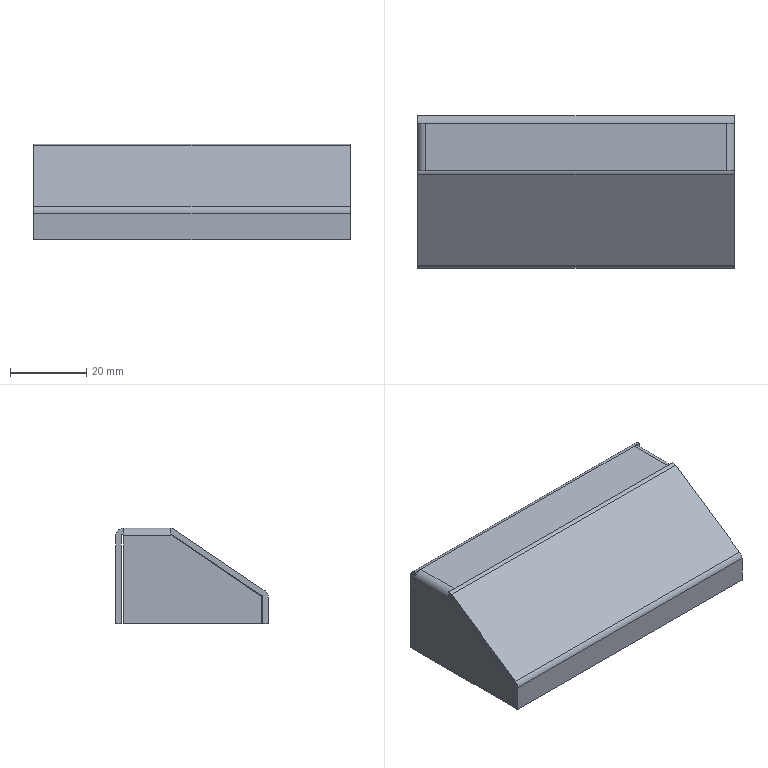Part | STEP file | Rear Door Handle 80 | 1 solid | 44 faces | box 83 x 40 x 25 mm | volume 11260 mm3 | plane 34 | cylinder 10 | commonest cylinder face diameters 1 x5 4 x5
STEP:
#1=CARTESIAN_POINT('',(83.,1.522,23.413));
#2=VERTEX_POINT('',#1);
#3=CARTESIAN_POINT('',(83.,-22.094,7.355));
#4=VERTEX_POINT('',#3);
#5=CARTESIAN_POINT('',(83.,2.031,23.76));
#6=DIRECTION('',(0.,-0.8269,-0.5623));
#7=VECTOR('',#6,1000.);
#8=LINE('',#5,#7);
#9=EDGE_CURVE('',#2,#4,#8,.T.);
#10=ORIENTED_EDGE('',*,*,#9,.T.);
#11=CARTESIAN_POINT('',(0.,-22.094,7.355));
#12=VERTEX_POINT('',#11);
#13=CARTESIAN_POINT('',(83.,-22.094,7.355));
#14=DIRECTION('',(-1.,0.,0.));
#15=VECTOR('',#14,1000.);
#16=LINE('',#13,#15);
#17=EDGE_CURVE('',#4,#12,#16,.T.);
#18=ORIENTED_EDGE('',*,*,#17,.T.);
#19=CARTESIAN_POINT('',(0.,1.522,23.413));
#20=VERTEX_POINT('',#19);
#21=CARTESIAN_POINT('',(0.,2.031,23.76));
#22=DIRECTION('',(0.,0.8269,0.5623));
#23=VECTOR('',#22,1000.);
#24=LINE('',#21,#23);
#25=EDGE_CURVE('',#12,#20,#24,.T.);
#26=ORIENTED_EDGE('',*,*,#25,.T.);
#27=CARTESIAN_POINT('',(83.,1.522,23.413));
#28=DIRECTION('',(1.,0.,0.));
#29=VECTOR('',#28,1000.);
#30=LINE('',#27,#29);
#31=EDGE_CURVE('',#20,#2,#30,.T.);
#32=ORIENTED_EDGE('',*,*,#31,.T.);
#33=EDGE_LOOP('',(#10,#18,#26,#32));
#34=FACE_OUTER_BOUND('',#33,.T.);
#35=CARTESIAN_POINT('',(83.,2.031,23.76));
#36=DIRECTION('',(0.,0.5623,-0.8269));
#37=DIRECTION('',(0.,0.8269,0.5623));
#38=AXIS2_PLACEMENT_3D('',#35,#36,#37);
#39=PLANE('',#38);
#40=ADVANCED_FACE('',(#34),#39,.T.);
#41=ORIENTED_EDGE('',*,*,#17,.F.);
#42=CARTESIAN_POINT('',(83.,-22.313,6.941));
#43=VERTEX_POINT('',#42);
#44=CARTESIAN_POINT('',(83.,-21.813,6.941));
#45=DIRECTION('',(-1.,0.,0.));
#46=DIRECTION('',(0.,0.,1.));
#47=AXIS2_PLACEMENT_3D('',#44,#45,#46);
#48=CIRCLE('',#47,0.5);
#49=EDGE_CURVE('',#43,#4,#48,.T.);
#50=ORIENTED_EDGE('',*,*,#49,.F.);
#51=CARTESIAN_POINT('',(0.,-22.313,6.941));
#52=VERTEX_POINT('',#51);
#53=CARTESIAN_POINT('',(83.,-22.313,6.941));
#54=DIRECTION('',(1.,0.,0.));
#55=VECTOR('',#54,1000.);
#56=LINE('',#53,#55);
#57=EDGE_CURVE('',#52,#43,#56,.T.);
#58=ORIENTED_EDGE('',*,*,#57,.F.);
#59=CARTESIAN_POINT('',(0.,-21.813,6.941));
#60=DIRECTION('',(1.,0.,0.));
#61=DIRECTION('',(0.,0.,1.));
#62=AXIS2_PLACEMENT_3D('',#59,#60,#61);
#63=CIRCLE('',#62,0.5);
#64=EDGE_CURVE('',#12,#52,#63,.T.);
#65=ORIENTED_EDGE('',*,*,#64,.F.);
#66=EDGE_LOOP('',(#41,#50,#58,#65));
#67=FACE_OUTER_BOUND('',#66,.T.);
#68=CARTESIAN_POINT('',(83.,-21.813,6.941));
#69=DIRECTION('',(-1.,0.,0.));
#70=DIRECTION('',(0.,0.,1.));
#71=AXIS2_PLACEMENT_3D('',#68,#69,#70);
#72=CYLINDRICAL_SURFACE('',#71,0.5);
#73=ADVANCED_FACE('',(#67),#72,.F.);
#74=ORIENTED_EDGE('',*,*,#9,.F.);
#75=CARTESIAN_POINT('',(83.,1.803,23.5));
#76=VERTEX_POINT('',#75);
#77=CARTESIAN_POINT('',(83.,1.803,23.));
#78=DIRECTION('',(-1.,0.,0.));
#79=DIRECTION('',(0.,0.,1.));
#80=AXIS2_PLACEMENT_3D('',#77,#78,#79);
#81=CIRCLE('',#80,0.5);
#82=EDGE_CURVE('',#2,#76,#81,.T.);
#83=ORIENTED_EDGE('',*,*,#82,.T.);
#84=CARTESIAN_POINT('',(83.,1.803,25.));
#85=VERTEX_POINT('',#84);
#86=CARTESIAN_POINT('',(83.,1.803,23.5));
#87=DIRECTION('',(0.,0.,-1.));
#88=VECTOR('',#87,1000.);
#89=LINE('',#86,#88);
#90=EDGE_CURVE('',#85,#76,#89,.T.);
#91=ORIENTED_EDGE('',*,*,#90,.F.);
#92=CARTESIAN_POINT('',(83.,0.6784,24.654));
#93=VERTEX_POINT('',#92);
#94=CARTESIAN_POINT('',(83.,1.803,23.));
#95=DIRECTION('',(-1.,0.,0.));
#96=DIRECTION('',(0.,0.,1.));
#97=AXIS2_PLACEMENT_3D('',#94,#95,#96);
#98=CIRCLE('',#97,2.);
#99=EDGE_CURVE('',#93,#85,#98,.T.);
#100=ORIENTED_EDGE('',*,*,#99,.F.);
#101=CARTESIAN_POINT('',(83.,-22.937,8.595));
#102=VERTEX_POINT('',#101);
#103=CARTESIAN_POINT('',(83.,0.6784,24.654));
#104=DIRECTION('',(0.,-0.8269,-0.5623));
#105=VECTOR('',#104,1000.);
#106=LINE('',#103,#105);
#107=EDGE_CURVE('',#93,#102,#106,.T.);
#108=ORIENTED_EDGE('',*,*,#107,.T.);
#109=CARTESIAN_POINT('',(83.,-23.813,6.941));
#110=VERTEX_POINT('',#109);
#111=CARTESIAN_POINT('',(83.,-21.813,6.941));
#112=DIRECTION('',(-1.,0.,0.));
#113=DIRECTION('',(0.,0.,1.));
#114=AXIS2_PLACEMENT_3D('',#111,#112,#113);
#115=CIRCLE('',#114,2.);
#116=EDGE_CURVE('',#110,#102,#115,.T.);
#117=ORIENTED_EDGE('',*,*,#116,.F.);
#118=CARTESIAN_POINT('',(83.,-23.813,0.));
#119=VERTEX_POINT('',#118);
#120=CARTESIAN_POINT('',(83.,-23.813,6.941));
#121=DIRECTION('',(0.,0.,-1.));
#122=VECTOR('',#121,1000.);
#123=LINE('',#120,#122);
#124=EDGE_CURVE('',#110,#119,#123,.T.);
#125=ORIENTED_EDGE('',*,*,#124,.T.);
#126=CARTESIAN_POINT('',(83.,-22.313,0.));
#127=VERTEX_POINT('',#126);
#128=CARTESIAN_POINT('',(83.,-22.313,0.));
#129=DIRECTION('',(0.,-1.,0.));
#130=VECTOR('',#129,1000.);
#131=LINE('',#128,#130);
#132=EDGE_CURVE('',#127,#119,#131,.T.);
#133=ORIENTED_EDGE('',*,*,#132,.F.);
#134=CARTESIAN_POINT('',(83.,-22.313,8.));
#135=DIRECTION('',(0.,0.,-1.));
#136=VECTOR('',#135,1000.);
#137=LINE('',#134,#136);
#138=EDGE_CURVE('',#43,#127,#137,.T.);
#139=ORIENTED_EDGE('',*,*,#138,.F.);
#140=ORIENTED_EDGE('',*,*,#49,.T.);
#141=EDGE_LOOP('',(#74,#83,#91,#100,#108,#117,#125,#133,#139,#140));
#142=FACE_OUTER_BOUND('',#141,.T.);
#143=CARTESIAN_POINT('',(83.,-22.313,6.941));
#144=DIRECTION('',(1.,0.,0.));
#145=DIRECTION('',(0.,0.,-1.));
#146=AXIS2_PLACEMENT_3D('',#143,#144,#145);
#147=PLANE('',#146);
#148=ADVANCED_FACE('',(#142),#147,.T.);
#149=CARTESIAN_POINT('',(0.06351,1.803,23.5));
#150=VERTEX_POINT('',#149);
#151=CARTESIAN_POINT('',(0.,1.803,23.5));
#152=VERTEX_POINT('',#151);
#153=CARTESIAN_POINT('',(2.,1.803,23.5));
#154=DIRECTION('',(-1.,0.,0.));
#155=VECTOR('',#154,1000.);
#156=LINE('',#153,#155);
#157=EDGE_CURVE('',#150,#152,#156,.T.);
#158=ORIENTED_EDGE('',*,*,#157,.F.);
#159=CARTESIAN_POINT('',(2.,1.803,23.5));
#160=VERTEX_POINT('',#159);
#161=CARTESIAN_POINT('',(83.,1.803,23.5));
#162=DIRECTION('',(-1.,0.,0.));
#163=VECTOR('',#162,1000.);
#164=LINE('',#161,#163);
#165=EDGE_CURVE('',#160,#150,#164,.T.);
#166=ORIENTED_EDGE('',*,*,#165,.F.);
#167=CARTESIAN_POINT('',(81.,1.803,23.5));
#168=VERTEX_POINT('',#167);
#169=CARTESIAN_POINT('',(83.,1.803,23.5));
#170=DIRECTION('',(-1.,0.,0.));
#171=VECTOR('',#170,1000.);
#172=LINE('',#169,#171);
#173=EDGE_CURVE('',#168,#160,#172,.T.);
#174=ORIENTED_EDGE('',*,*,#173,.F.);
#175=CARTESIAN_POINT('',(82.936,1.803,23.5));
#176=VERTEX_POINT('',#175);
#177=CARTESIAN_POINT('',(83.,1.803,23.5));
#178=DIRECTION('',(-1.,0.,0.));
#179=VECTOR('',#178,1000.);
#180=LINE('',#177,#179);
#181=EDGE_CURVE('',#176,#168,#180,.T.);
#182=ORIENTED_EDGE('',*,*,#181,.F.);
#183=CARTESIAN_POINT('',(83.,1.803,23.5));
#184=DIRECTION('',(-1.,0.,0.));
#185=VECTOR('',#184,1000.);
#186=LINE('',#183,#185);
#187=EDGE_CURVE('',#76,#176,#186,.T.);
#188=ORIENTED_EDGE('',*,*,#187,.F.);
#189=ORIENTED_EDGE('',*,*,#82,.F.);
#190=ORIENTED_EDGE('',*,*,#31,.F.);
#191=CARTESIAN_POINT('',(0.,1.803,23.));
#192=DIRECTION('',(1.,0.,0.));
#193=DIRECTION('',(0.,0.,1.));
#194=AXIS2_PLACEMENT_3D('',#191,#192,#193);
#195=CIRCLE('',#194,0.5);
#196=EDGE_CURVE('',#152,#20,#195,.T.);
#197=ORIENTED_EDGE('',*,*,#196,.F.);
#198=EDGE_LOOP('',(#158,#166,#174,#182,#188,#189,#190,#197));
#199=FACE_OUTER_BOUND('',#198,.T.);
#200=CARTESIAN_POINT('',(83.,1.803,23.));
#201=DIRECTION('',(-1.,0.,0.));
#202=DIRECTION('',(0.,0.,1.));
#203=AXIS2_PLACEMENT_3D('',#200,#201,#202);
#204=CYLINDRICAL_SURFACE('',#203,0.5);
#205=ADVANCED_FACE('',(#199),#204,.F.);
#206=ORIENTED_EDGE('',*,*,#25,.F.);
#207=ORIENTED_EDGE('',*,*,#64,.T.);
#208=CARTESIAN_POINT('',(0.,-22.313,0.));
#209=VERTEX_POINT('',#208);
#210=CARTESIAN_POINT('',(0.,-22.313,8.));
#211=DIRECTION('',(0.,0.,1.));
#212=VECTOR('',#211,1000.);
#213=LINE('',#210,#212);
#214=EDGE_CURVE('',#209,#52,#213,.T.);
#215=ORIENTED_EDGE('',*,*,#214,.F.);
#216=CARTESIAN_POINT('',(0.,-23.813,0.));
#217=VERTEX_POINT('',#216);
#218=CARTESIAN_POINT('',(0.,-22.313,0.));
#219=DIRECTION('',(0.,1.,0.));
#220=VECTOR('',#219,1000.);
#221=LINE('',#218,#220);
#222=EDGE_CURVE('',#217,#209,#221,.T.);
#223=ORIENTED_EDGE('',*,*,#222,.F.);
#224=CARTESIAN_POINT('',(0.,-23.813,6.941));
#225=VERTEX_POINT('',#224);
#226=CARTESIAN_POINT('',(0.,-23.813,7.355));
#227=DIRECTION('',(0.,0.,1.));
#228=VECTOR('',#227,1000.);
#229=LINE('',#226,#228);
#230=EDGE_CURVE('',#217,#225,#229,.T.);
#231=ORIENTED_EDGE('',*,*,#230,.T.);
#232=CARTESIAN_POINT('',(0.,-22.937,8.595));
#233=VERTEX_POINT('',#232);
#234=CARTESIAN_POINT('',(0.,-21.813,6.941));
#235=DIRECTION('',(1.,0.,0.));
#236=DIRECTION('',(0.,0.,1.));
#237=AXIS2_PLACEMENT_3D('',#234,#235,#236);
#238=CIRCLE('',#237,2.);
#239=EDGE_CURVE('',#233,#225,#238,.T.);
#240=ORIENTED_EDGE('',*,*,#239,.F.);
#241=CARTESIAN_POINT('',(0.,0.6784,24.654));
#242=VERTEX_POINT('',#241);
#243=CARTESIAN_POINT('',(0.,-22.937,8.595));
#244=DIRECTION('',(0.,0.8269,0.5623));
#245=VECTOR('',#244,1000.);
#246=LINE('',#243,#245);
#247=EDGE_CURVE('',#233,#242,#246,.T.);
#248=ORIENTED_EDGE('',*,*,#247,.T.);
#249=CARTESIAN_POINT('',(0.,1.803,25.));
#250=VERTEX_POINT('',#249);
#251=CARTESIAN_POINT('',(0.,1.803,23.));
#252=DIRECTION('',(-1.,0.,0.));
#253=DIRECTION('',(0.,0.,1.));
#254=AXIS2_PLACEMENT_3D('',#251,#252,#253);
#255=CIRCLE('',#254,2.);
#256=EDGE_CURVE('',#242,#250,#255,.T.);
#257=ORIENTED_EDGE('',*,*,#256,.T.);
#258=CARTESIAN_POINT('',(0.,1.803,23.5));
#259=DIRECTION('',(0.,0.,1.));
#260=VECTOR('',#259,1000.);
#261=LINE('',#258,#260);
#262=EDGE_CURVE('',#152,#250,#261,.T.);
#263=ORIENTED_EDGE('',*,*,#262,.F.);
#264=ORIENTED_EDGE('',*,*,#196,.T.);
#265=EDGE_LOOP('',(#206,#207,#215,#223,#231,#240,#248,#257,#263,#264));
#266=FACE_OUTER_BOUND('',#265,.T.);
#267=CARTESIAN_POINT('',(0.,1.803,23.5));
#268=DIRECTION('',(-1.,0.,0.));
#269=DIRECTION('',(0.,0.,1.));
#270=AXIS2_PLACEMENT_3D('',#267,#268,#269);
#271=PLANE('',#270);
#272=ADVANCED_FACE('',(#266),#271,.T.);
#273=ORIENTED_EDGE('',*,*,#138,.T.);
#274=CARTESIAN_POINT('',(83.,-22.313,0.));
#275=DIRECTION('',(-1.,0.,0.));
#276=VECTOR('',#275,1000.);
#277=LINE('',#274,#276);
#278=EDGE_CURVE('',#127,#209,#277,.T.);
#279=ORIENTED_EDGE('',*,*,#278,.T.);
#280=ORIENTED_EDGE('',*,*,#214,.T.);
#281=ORIENTED_EDGE('',*,*,#57,.T.);
#282=EDGE_LOOP('',(#273,#279,#280,#281));
#283=FACE_OUTER_BOUND('',#282,.T.);
#284=CARTESIAN_POINT('',(83.,-22.313,8.));
#285=DIRECTION('',(0.,1.,0.));
#286=DIRECTION('',(0.,0.,1.));
#287=AXIS2_PLACEMENT_3D('',#284,#285,#286);
#288=PLANE('',#287);
#289=ADVANCED_FACE('',(#283),#288,.T.);
#290=CARTESIAN_POINT('',(83.,-22.937,8.595));
#291=DIRECTION('',(-1.,0.,0.));
#292=VECTOR('',#291,1000.);
#293=LINE('',#290,#292);
#294=EDGE_CURVE('',#102,#233,#293,.T.);
#295=ORIENTED_EDGE('',*,*,#294,.F.);
#296=ORIENTED_EDGE('',*,*,#107,.F.);
#297=CARTESIAN_POINT('',(83.,0.6784,24.654));
#298=DIRECTION('',(1.,0.,0.));
#299=VECTOR('',#298,1000.);
#300=LINE('',#297,#299);
#301=EDGE_CURVE('',#242,#93,#300,.T.);
#302=ORIENTED_EDGE('',*,*,#301,.F.);
#303=ORIENTED_EDGE('',*,*,#247,.F.);
#304=EDGE_LOOP('',(#295,#296,#302,#303));
#305=FACE_OUTER_BOUND('',#304,.T.);
#306=CARTESIAN_POINT('',(83.,1.187,25.));
#307=DIRECTION('',(0.,0.5623,-0.8269));
#308=DIRECTION('',(0.,0.8269,0.5623));
#309=AXIS2_PLACEMENT_3D('',#306,#307,#308);
#310=PLANE('',#309);
#311=ADVANCED_FACE('',(#305),#310,.F.);
#312=CARTESIAN_POINT('',(0.,1.803,23.));
#313=VERTEX_POINT('',#312);
#314=CARTESIAN_POINT('',(2.,1.803,23.));
#315=DIRECTION('',(0.,1.,0.));
#316=DIRECTION('',(0.,0.,1.));
#317=AXIS2_PLACEMENT_3D('',#314,#315,#316);
#318=CIRCLE('',#317,2.);
#319=EDGE_CURVE('',#313,#150,#318,.T.);
#320=ORIENTED_EDGE('',*,*,#319,.F.);
#321=CARTESIAN_POINT('',(1.5,1.803,23.));
#322=VERTEX_POINT('',#321);
#323=CARTESIAN_POINT('',(2.,1.803,23.));
#324=DIRECTION('',(1.,0.,0.));
#325=VECTOR('',#324,1000.);
#326=LINE('',#323,#325);
#327=EDGE_CURVE('',#313,#322,#326,.T.);
#328=ORIENTED_EDGE('',*,*,#327,.T.);
#329=CARTESIAN_POINT('',(2.,1.803,23.));
#330=DIRECTION('',(0.,1.,0.));
#331=DIRECTION('',(0.,0.,1.));
#332=AXIS2_PLACEMENT_3D('',#329,#330,#331);
#333=CIRCLE('',#332,0.5);
#334=EDGE_CURVE('',#322,#160,#333,.T.);
#335=ORIENTED_EDGE('',*,*,#334,.T.);
#336=ORIENTED_EDGE('',*,*,#165,.T.);
#337=EDGE_LOOP('',(#320,#328,#335,#336));
#338=FACE_OUTER_BOUND('',#337,.T.);
#339=CARTESIAN_POINT('',(2.,1.803,23.));
#340=DIRECTION('',(0.,-1.,0.));
#341=DIRECTION('',(0.,0.,-1.));
#342=AXIS2_PLACEMENT_3D('',#339,#340,#341);
#343=PLANE('',#342);
#344=ADVANCED_FACE('',(#338),#343,.T.);
#345=CARTESIAN_POINT('',(2.,14.187,23.5));
#346=VERTEX_POINT('',#345);
#347=CARTESIAN_POINT('',(81.,14.187,23.5));
#348=VERTEX_POINT('',#347);
#349=CARTESIAN_POINT('',(83.,14.187,23.5));
#350=DIRECTION('',(1.,0.,0.));
#351=VECTOR('',#350,1000.);
#352=LINE('',#349,#351);
#353=EDGE_CURVE('',#346,#348,#352,.T.);
#354=ORIENTED_EDGE('',*,*,#353,.T.);
#355=CARTESIAN_POINT('',(81.,16.187,23.5));
#356=DIRECTION('',(0.,-1.,0.));
#357=VECTOR('',#356,1000.);
#358=LINE('',#355,#357);
#359=EDGE_CURVE('',#348,#168,#358,.T.);
#360=ORIENTED_EDGE('',*,*,#359,.T.);
#361=ORIENTED_EDGE('',*,*,#173,.T.);
#362=CARTESIAN_POINT('',(2.,16.187,23.5));
#363=DIRECTION('',(0.,1.,0.));
#364=VECTOR('',#363,1000.);
#365=LINE('',#362,#364);
#366=EDGE_CURVE('',#160,#346,#365,.T.);
#367=ORIENTED_EDGE('',*,*,#366,.T.);
#368=EDGE_LOOP('',(#354,#360,#361,#367));
#369=FACE_OUTER_BOUND('',#368,.T.);
#370=CARTESIAN_POINT('',(83.,16.187,23.5));
#371=DIRECTION('',(0.,0.,-1.));
#372=DIRECTION('',(-1.,0.,0.));
#373=AXIS2_PLACEMENT_3D('',#370,#371,#372);
#374=PLANE('',#373);
#375=ADVANCED_FACE('',(#369),#374,.T.);
#376=ORIENTED_EDGE('',*,*,#181,.T.);
#377=CARTESIAN_POINT('',(81.5,1.803,23.));
#378=VERTEX_POINT('',#377);
#379=CARTESIAN_POINT('',(81.,1.803,23.));
#380=DIRECTION('',(0.,-1.,0.));
#381=DIRECTION('',(0.,0.,-1.));
#382=AXIS2_PLACEMENT_3D('',#379,#380,#381);
#383=CIRCLE('',#382,0.5);
#384=EDGE_CURVE('',#378,#168,#383,.T.);
#385=ORIENTED_EDGE('',*,*,#384,.F.);
#386=CARTESIAN_POINT('',(83.,1.803,23.));
#387=VERTEX_POINT('',#386);
#388=CARTESIAN_POINT('',(81.,1.803,23.));
#389=DIRECTION('',(-1.,0.,0.));
#390=VECTOR('',#389,1000.);
#391=LINE('',#388,#390);
#392=EDGE_CURVE('',#387,#378,#391,.T.);
#393=ORIENTED_EDGE('',*,*,#392,.F.);
#394=CARTESIAN_POINT('',(81.,1.803,23.));
#395=DIRECTION('',(0.,1.,0.));
#396=DIRECTION('',(0.,0.,-1.));
#397=AXIS2_PLACEMENT_3D('',#394,#395,#396);
#398=CIRCLE('',#397,2.);
#399=EDGE_CURVE('',#176,#387,#398,.T.);
#400=ORIENTED_EDGE('',*,*,#399,.F.);
#401=EDGE_LOOP('',(#376,#385,#393,#400));
#402=FACE_OUTER_BOUND('',#401,.T.);
#403=CARTESIAN_POINT('',(81.,1.803,23.));
#404=DIRECTION('',(0.,1.,0.));
#405=DIRECTION('',(0.,0.,1.));
#406=AXIS2_PLACEMENT_3D('',#403,#404,#405);
#407=PLANE('',#406);
#408=ADVANCED_FACE('',(#402),#407,.F.);
#409=ORIENTED_EDGE('',*,*,#132,.T.);
#410=CARTESIAN_POINT('',(83.,-23.813,0.));
#411=DIRECTION('',(-1.,0.,0.));
#412=VECTOR('',#411,1000.);
#413=LINE('',#410,#412);
#414=EDGE_CURVE('',#119,#217,#413,.T.);
#415=ORIENTED_EDGE('',*,*,#414,.T.);
#416=ORIENTED_EDGE('',*,*,#222,.T.);
#417=ORIENTED_EDGE('',*,*,#278,.F.);
#418=EDGE_LOOP('',(#409,#415,#416,#417));
#419=FACE_OUTER_BOUND('',#418,.T.);
#420=CARTESIAN_POINT('',(83.,-22.313,0.));
#421=DIRECTION('',(0.,0.,-1.));
#422=DIRECTION('',(-1.,0.,0.));
#423=AXIS2_PLACEMENT_3D('',#420,#421,#422);
#424=PLANE('',#423);
#425=ADVANCED_FACE('',(#419),#424,.T.);
#426=ORIENTED_EDGE('',*,*,#116,.T.);
#427=ORIENTED_EDGE('',*,*,#294,.T.);
#428=ORIENTED_EDGE('',*,*,#239,.T.);
#429=CARTESIAN_POINT('',(83.,-23.813,6.941));
#430=DIRECTION('',(1.,0.,0.));
#431=VECTOR('',#430,1000.);
#432=LINE('',#429,#431);
#433=EDGE_CURVE('',#225,#110,#432,.T.);
#434=ORIENTED_EDGE('',*,*,#433,.T.);
#435=EDGE_LOOP('',(#426,#427,#428,#434));
#436=FACE_OUTER_BOUND('',#435,.T.);
#437=CARTESIAN_POINT('',(83.,-21.813,6.941));
#438=DIRECTION('',(-1.,0.,0.));
#439=DIRECTION('',(0.,0.,1.));
#440=AXIS2_PLACEMENT_3D('',#437,#438,#439);
#441=CYLINDRICAL_SURFACE('',#440,2.);
#442=ADVANCED_FACE('',(#436),#441,.T.);
#443=CARTESIAN_POINT('',(81.,1.803,25.));
#444=VERTEX_POINT('',#443);
#445=CARTESIAN_POINT('',(2.,1.803,25.));
#446=VERTEX_POINT('',#445);
#447=CARTESIAN_POINT('',(83.,1.803,25.));
#448=DIRECTION('',(-1.,0.,0.));
#449=VECTOR('',#448,1000.);
#450=LINE('',#447,#449);
#451=EDGE_CURVE('',#444,#446,#450,.T.);
#452=ORIENTED_EDGE('',*,*,#451,.T.);
#453=CARTESIAN_POINT('',(83.,1.803,25.));
#454=DIRECTION('',(-1.,0.,0.));
#455=VECTOR('',#454,1000.);
#456=LINE('',#453,#455);
#457=EDGE_CURVE('',#446,#250,#456,.T.);
#458=ORIENTED_EDGE('',*,*,#457,.T.);
#459=ORIENTED_EDGE('',*,*,#256,.F.);
#460=ORIENTED_EDGE('',*,*,#301,.T.);
#461=ORIENTED_EDGE('',*,*,#99,.T.);
#462=CARTESIAN_POINT('',(83.,1.803,25.));
#463=DIRECTION('',(-1.,0.,0.));
#464=VECTOR('',#463,1000.);
#465=LINE('',#462,#464);
#466=EDGE_CURVE('',#85,#444,#465,.T.);
#467=ORIENTED_EDGE('',*,*,#466,.T.);
#468=EDGE_LOOP('',(#452,#458,#459,#460,#461,#467));
#469=FACE_OUTER_BOUND('',#468,.T.);
#470=CARTESIAN_POINT('',(83.,1.803,23.));
#471=DIRECTION('',(-1.,0.,0.));
#472=DIRECTION('',(0.,0.,1.));
#473=AXIS2_PLACEMENT_3D('',#470,#471,#472);
#474=CYLINDRICAL_SURFACE('',#473,2.);
#475=ADVANCED_FACE('',(#469),#474,.T.);
#476=CARTESIAN_POINT('',(1.5,1.634,23.248));
#477=VERTEX_POINT('',#476);
#478=CARTESIAN_POINT('',(1.5,1.803,23.));
#479=DIRECTION('',(0.,-0.5623,0.8269));
#480=VECTOR('',#479,1000.);
#481=LINE('',#478,#480);
#482=EDGE_CURVE('',#322,#477,#481,.T.);
#483=ORIENTED_EDGE('',*,*,#482,.F.);
#484=ORIENTED_EDGE('',*,*,#327,.F.);
#485=CARTESIAN_POINT('',(0.,1.634,23.248));
#486=VERTEX_POINT('',#485);
#487=CARTESIAN_POINT('',(0.,1.803,23.));
#488=DIRECTION('',(0.,-0.5623,0.8269));
#489=VECTOR('',#488,1000.);
#490=LINE('',#487,#489);
#491=EDGE_CURVE('',#313,#486,#490,.T.);
#492=ORIENTED_EDGE('',*,*,#491,.T.);
#493=CARTESIAN_POINT('',(1.5,1.634,23.248));
#494=DIRECTION('',(-1.,0.,0.));
#495=VECTOR('',#494,1000.);
#496=LINE('',#493,#495);
#497=EDGE_CURVE('',#477,#486,#496,.T.);
#498=ORIENTED_EDGE('',*,*,#497,.F.);
#499=EDGE_LOOP('',(#483,#484,#492,#498));
#500=FACE_OUTER_BOUND('',#499,.T.);
#501=CARTESIAN_POINT('',(1.5,1.803,23.));
#502=DIRECTION('',(0.,0.8269,0.5623));
#503=DIRECTION('',(0.,-0.5623,0.8269));
#504=AXIS2_PLACEMENT_3D('',#501,#502,#503);
#505=PLANE('',#504);
#506=ADVANCED_FACE('',(#500),#505,.T.);
#507=CARTESIAN_POINT('',(81.5,14.187,23.));
#508=VERTEX_POINT('',#507);
#509=CARTESIAN_POINT('',(81.,14.187,23.));
#510=DIRECTION('',(0.,-1.,0.));
#511=DIRECTION('',(0.,0.,-1.));
#512=AXIS2_PLACEMENT_3D('',#509,#510,#511);
#513=CIRCLE('',#512,0.5);
#514=EDGE_CURVE('',#508,#348,#513,.T.);
#515=ORIENTED_EDGE('',*,*,#514,.F.);
#516=CARTESIAN_POINT('',(81.5,1.803,23.));
#517=DIRECTION('',(0.,1.,0.));
#518=VECTOR('',#517,1000.);
#519=LINE('',#516,#518);
#520=EDGE_CURVE('',#378,#508,#519,.T.);
#521=ORIENTED_EDGE('',*,*,#520,.F.);
#522=ORIENTED_EDGE('',*,*,#384,.T.);
#523=ORIENTED_EDGE('',*,*,#359,.F.);
#524=EDGE_LOOP('',(#515,#521,#522,#523));
#525=FACE_OUTER_BOUND('',#524,.T.);
#526=CARTESIAN_POINT('',(81.,1.803,23.));
#527=DIRECTION('',(0.,-1.,0.));
#528=DIRECTION('',(0.,0.,-1.));
#529=AXIS2_PLACEMENT_3D('',#526,#527,#528);
#530=CYLINDRICAL_SURFACE('',#529,0.5);
#531=ADVANCED_FACE('',(#525),#530,.F.);
#532=CARTESIAN_POINT('',(83.,14.687,23.));
#533=VERTEX_POINT('',#532);
#534=CARTESIAN_POINT('',(0.,14.687,23.));
#535=VERTEX_POINT('',#534);
#536=CARTESIAN_POINT('',(83.,14.687,23.));
#537=DIRECTION('',(-1.,0.,0.));
#538=VECTOR('',#537,1000.);
#539=LINE('',#536,#538);
#540=EDGE_CURVE('',#533,#535,#539,.T.);
#541=ORIENTED_EDGE('',*,*,#540,.F.);
#542=CARTESIAN_POINT('',(83.,14.187,23.5));
#543=VERTEX_POINT('',#542);
#544=CARTESIAN_POINT('',(83.,14.187,23.));
#545=DIRECTION('',(-1.,0.,0.));
#546=DIRECTION('',(0.,0.,1.));
#547=AXIS2_PLACEMENT_3D('',#544,#545,#546);
#548=CIRCLE('',#547,0.5);
#549=EDGE_CURVE('',#543,#533,#548,.T.);
#550=ORIENTED_EDGE('',*,*,#549,.F.);
#551=CARTESIAN_POINT('',(82.936,14.187,23.5));
#552=VERTEX_POINT('',#551);
#553=CARTESIAN_POINT('',(81.,14.187,23.5));
#554=DIRECTION('',(1.,0.,0.));
#555=VECTOR('',#554,1000.);
#556=LINE('',#553,#555);
#557=EDGE_CURVE('',#552,#543,#556,.T.);
#558=ORIENTED_EDGE('',*,*,#557,.F.);
#559=CARTESIAN_POINT('',(83.,14.187,23.5));
#560=DIRECTION('',(1.,0.,0.));
#561=VECTOR('',#560,1000.);
#562=LINE('',#559,#561);
#563=EDGE_CURVE('',#348,#552,#562,.T.);
#564=ORIENTED_EDGE('',*,*,#563,.F.);
#565=ORIENTED_EDGE('',*,*,#353,.F.);
#566=CARTESIAN_POINT('',(0.06351,14.187,23.5));
#567=VERTEX_POINT('',#566);
#568=CARTESIAN_POINT('',(83.,14.187,23.5));
#569=DIRECTION('',(1.,0.,0.));
#570=VECTOR('',#569,1000.);
#571=LINE('',#568,#570);
#572=EDGE_CURVE('',#567,#346,#571,.T.);
#573=ORIENTED_EDGE('',*,*,#572,.F.);
#574=CARTESIAN_POINT('',(0.,14.187,23.5));
#575=VERTEX_POINT('',#574);
#576=CARTESIAN_POINT('',(0.,14.187,23.5));
#577=DIRECTION('',(1.,0.,0.));
#578=VECTOR('',#577,1000.);
#579=LINE('',#576,#578);
#580=EDGE_CURVE('',#575,#567,#579,.T.);
#581=ORIENTED_EDGE('',*,*,#580,.F.);
#582=CARTESIAN_POINT('',(0.,14.187,23.));
#583=DIRECTION('',(1.,0.,0.));
#584=DIRECTION('',(0.,0.,1.));
#585=AXIS2_PLACEMENT_3D('',#582,#583,#584);
#586=CIRCLE('',#585,0.5);
#587=EDGE_CURVE('',#535,#575,#586,.T.);
#588=ORIENTED_EDGE('',*,*,#587,.F.);
#589=EDGE_LOOP('',(#541,#550,#558,#564,#565,#573,#581,#588));
#590=FACE_OUTER_BOUND('',#589,.T.);
#591=CARTESIAN_POINT('',(83.,14.187,23.));
#592=DIRECTION('',(-1.,0.,0.));
#593=DIRECTION('',(0.,0.,1.));
#594=AXIS2_PLACEMENT_3D('',#591,#592,#593);
#595=CYLINDRICAL_SURFACE('',#594,0.5);
#596=ADVANCED_FACE('',(#590),#595,.F.);
#597=ORIENTED_EDGE('',*,*,#334,.F.);
#598=CARTESIAN_POINT('',(1.5,14.187,23.));
#599=VERTEX_POINT('',#598);
#600=CARTESIAN_POINT('',(1.5,14.187,23.));
#601=DIRECTION('',(0.,-1.,0.));
#602=VECTOR('',#601,1000.);
#603=LINE('',#600,#602);
#604=EDGE_CURVE('',#599,#322,#603,.T.);
#605=ORIENTED_EDGE('',*,*,#604,.F.);
#606=CARTESIAN_POINT('',(2.,14.187,23.));
#607=DIRECTION('',(0.,-1.,0.));
#608=DIRECTION('',(0.,0.,1.));
#609=AXIS2_PLACEMENT_3D('',#606,#607,#608);
#610=CIRCLE('',#609,0.5);
#611=EDGE_CURVE('',#346,#599,#610,.T.);
#612=ORIENTED_EDGE('',*,*,#611,.F.);
#613=ORIENTED_EDGE('',*,*,#366,.F.);
#614=EDGE_LOOP('',(#597,#605,#612,#613));
#615=FACE_OUTER_BOUND('',#614,.T.);
#616=CARTESIAN_POINT('',(2.,14.187,23.));
#617=DIRECTION('',(0.,1.,0.));
#618=DIRECTION('',(0.,0.,1.));
#619=AXIS2_PLACEMENT_3D('',#616,#617,#618);
#620=CYLINDRICAL_SURFACE('',#619,0.5);
#621=ADVANCED_FACE('',(#615),#620,.F.);
#622=CARTESIAN_POINT('',(81.5,1.634,23.248));
#623=VERTEX_POINT('',#622);
#624=CARTESIAN_POINT('',(81.5,1.803,23.));
#625=DIRECTION('',(0.,-0.5623,0.8269));
#626=VECTOR('',#625,1000.);
#627=LINE('',#624,#626);
#628=EDGE_CURVE('',#378,#623,#627,.T.);
#629=ORIENTED_EDGE('',*,*,#628,.T.);
#630=CARTESIAN_POINT('',(83.,1.634,23.248));
#631=VERTEX_POINT('',#630);
#632=CARTESIAN_POINT('',(81.5,1.634,23.248));
#633=DIRECTION('',(-1.,0.,0.));
#634=VECTOR('',#633,1000.);
#635=LINE('',#632,#634);
#636=EDGE_CURVE('',#631,#623,#635,.T.);
#637=ORIENTED_EDGE('',*,*,#636,.F.);
#638=CARTESIAN_POINT('',(83.,1.803,23.));
#639=DIRECTION('',(0.,-0.5623,0.8269));
#640=VECTOR('',#639,1000.);
#641=LINE('',#638,#640);
#642=EDGE_CURVE('',#387,#631,#641,.T.);
#643=ORIENTED_EDGE('',*,*,#642,.F.);
#644=ORIENTED_EDGE('',*,*,#392,.T.);
#645=EDGE_LOOP('',(#629,#637,#643,#644));
#646=FACE_OUTER_BOUND('',#645,.T.);
#647=CARTESIAN_POINT('',(81.5,1.803,23.));
#648=DIRECTION('',(0.,0.8269,0.5623));
#649=DIRECTION('',(0.,-0.5623,0.8269));
#650=AXIS2_PLACEMENT_3D('',#647,#648,#649);
#651=PLANE('',#650);
#652=ADVANCED_FACE('',(#646),#651,.T.);
#653=ORIENTED_EDGE('',*,*,#414,.F.);
#654=ORIENTED_EDGE('',*,*,#124,.F.);
#655=ORIENTED_EDGE('',*,*,#433,.F.);
#656=ORIENTED_EDGE('',*,*,#230,.F.);
#657=EDGE_LOOP('',(#653,#654,#655,#656));
#658=FACE_OUTER_BOUND('',#657,.T.);
#659=CARTESIAN_POINT('',(83.,-23.813,8.));
#660=DIRECTION('',(0.,1.,0.));
#661=DIRECTION('',(0.,0.,1.));
#662=AXIS2_PLACEMENT_3D('',#659,#660,#661);
#663=PLANE('',#662);
#664=ADVANCED_FACE('',(#658),#663,.F.);
#665=ORIENTED_EDGE('',*,*,#157,.T.);
#666=ORIENTED_EDGE('',*,*,#262,.T.);
#667=ORIENTED_EDGE('',*,*,#457,.F.);
#668=CARTESIAN_POINT('',(2.,1.803,23.));
#669=DIRECTION('',(0.,-1.,0.));
#670=DIRECTION('',(0.,0.,1.));
#671=AXIS2_PLACEMENT_3D('',#668,#669,#670);
#672=CIRCLE('',#671,2.);
#673=EDGE_CURVE('',#446,#150,#672,.T.);
#674=ORIENTED_EDGE('',*,*,#673,.T.);
#675=EDGE_LOOP('',(#665,#666,#667,#674));
#676=FACE_OUTER_BOUND('',#675,.T.);
#677=CARTESIAN_POINT('',(2.,1.803,23.5));
#678=DIRECTION('',(0.,1.,0.));
#679=DIRECTION('',(-1.,0.,0.));
#680=AXIS2_PLACEMENT_3D('',#677,#678,#679);
#681=PLANE('',#680);
#682=ADVANCED_FACE('',(#676),#681,.T.);
#683=ORIENTED_EDGE('',*,*,#451,.F.);
#684=CARTESIAN_POINT('',(81.,14.187,25.));
#685=VERTEX_POINT('',#684);
#686=CARTESIAN_POINT('',(81.,16.187,25.));
#687=DIRECTION('',(0.,-1.,0.));
#688=VECTOR('',#687,1000.);
#689=LINE('',#686,#688);
#690=EDGE_CURVE('',#685,#444,#689,.T.);
#691=ORIENTED_EDGE('',*,*,#690,.F.);
#692=CARTESIAN_POINT('',(2.,14.187,25.));
#693=VERTEX_POINT('',#692);
#694=CARTESIAN_POINT('',(83.,14.187,25.));
#695=DIRECTION('',(1.,0.,0.));
#696=VECTOR('',#695,1000.);
#697=LINE('',#694,#696);
#698=EDGE_CURVE('',#693,#685,#697,.T.);
#699=ORIENTED_EDGE('',*,*,#698,.F.);
#700=CARTESIAN_POINT('',(2.,16.187,25.));
#701=DIRECTION('',(0.,1.,0.));
#702=VECTOR('',#701,1000.);
#703=LINE('',#700,#702);
#704=EDGE_CURVE('',#446,#693,#703,.T.);
#705=ORIENTED_EDGE('',*,*,#704,.F.);
#706=EDGE_LOOP('',(#683,#691,#699,#705));
#707=FACE_OUTER_BOUND('',#706,.T.);
#708=CARTESIAN_POINT('',(83.,16.187,25.));
#709=DIRECTION('',(0.,0.,-1.));
#710=DIRECTION('',(-1.,0.,0.));
#711=AXIS2_PLACEMENT_3D('',#708,#709,#710);
#712=PLANE('',#711);
#713=ADVANCED_FACE('',(#707),#712,.F.);
#714=ORIENTED_EDGE('',*,*,#466,.F.);
#715=ORIENTED_EDGE('',*,*,#90,.T.);
#716=ORIENTED_EDGE('',*,*,#187,.T.);
#717=CARTESIAN_POINT('',(81.,1.803,23.));
#718=DIRECTION('',(0.,-1.,0.));
#719=DIRECTION('',(0.,0.,-1.));
#720=AXIS2_PLACEMENT_3D('',#717,#718,#719);
#721=CIRCLE('',#720,2.);
#722=EDGE_CURVE('',#176,#444,#721,.T.);
#723=ORIENTED_EDGE('',*,*,#722,.T.);
#724=EDGE_LOOP('',(#714,#715,#716,#723));
#725=FACE_OUTER_BOUND('',#724,.T.);
#726=CARTESIAN_POINT('',(83.,1.803,23.5));
#727=DIRECTION('',(0.,1.,0.));
#728=DIRECTION('',(-1.,0.,0.));
#729=AXIS2_PLACEMENT_3D('',#726,#727,#728);
#730=PLANE('',#729);
#731=ADVANCED_FACE('',(#725),#730,.T.);
#732=CARTESIAN_POINT('',(81.5,14.187,0.));
#733=VERTEX_POINT('',#732);
#734=CARTESIAN_POINT('',(81.5,14.187,0.));
#735=DIRECTION('',(0.,0.,1.));
#736=VECTOR('',#735,1000.);
#737=LINE('',#734,#736);
#738=EDGE_CURVE('',#733,#508,#737,.T.);
#739=ORIENTED_EDGE('',*,*,#738,.F.);
#740=CARTESIAN_POINT('',(81.5,-22.113,0.));
#741=VERTEX_POINT('',#740);
#742=CARTESIAN_POINT('',(81.5,0.,0.));
#743=DIRECTION('',(0.,1.,0.));
#744=VECTOR('',#743,1000.);
#745=LINE('',#742,#744);
#746=EDGE_CURVE('',#741,#733,#745,.T.);
#747=ORIENTED_EDGE('',*,*,#746,.F.);
#748=CARTESIAN_POINT('',(81.5,-22.113,7.1));
#749=VERTEX_POINT('',#748);
#750=CARTESIAN_POINT('',(81.5,-22.113,0.));
#751=DIRECTION('',(0.,0.,-1.));
#752=VECTOR('',#751,1000.);
#753=LINE('',#750,#752);
#754=EDGE_CURVE('',#749,#741,#753,.T.);
#755=ORIENTED_EDGE('',*,*,#754,.F.);
#756=CARTESIAN_POINT('',(81.5,1.634,23.248));
#757=DIRECTION('',(0.,-0.8269,-0.5623));
#758=VECTOR('',#757,1000.);
#759=LINE('',#756,#758);
#760=EDGE_CURVE('',#623,#749,#759,.T.);
#761=ORIENTED_EDGE('',*,*,#760,.F.);
#762=ORIENTED_EDGE('',*,*,#628,.F.);
#763=ORIENTED_EDGE('',*,*,#520,.T.);
#764=EDGE_LOOP('',(#739,#747,#755,#761,#762,#763));
#765=FACE_OUTER_BOUND('',#764,.T.);
#766=CARTESIAN_POINT('',(81.5,0.,0.));
#767=DIRECTION('',(1.,0.,0.));
#768=DIRECTION('',(0.,0.,-1.));
#769=AXIS2_PLACEMENT_3D('',#766,#767,#768);
#770=PLANE('',#769);
#771=ADVANCED_FACE('',(#765),#770,.F.);
#772=CARTESIAN_POINT('',(83.,14.687,0.));
#773=VERTEX_POINT('',#772);
#774=CARTESIAN_POINT('',(83.,14.687,0.));
#775=DIRECTION('',(0.,0.,1.));
#776=VECTOR('',#775,1000.);
#777=LINE('',#774,#776);
#778=EDGE_CURVE('',#773,#533,#777,.T.);
#779=ORIENTED_EDGE('',*,*,#778,.T.);
#780=ORIENTED_EDGE('',*,*,#540,.T.);
#781=CARTESIAN_POINT('',(0.,14.687,0.));
#782=VERTEX_POINT('',#781);
#783=CARTESIAN_POINT('',(0.,14.687,0.));
#784=DIRECTION('',(0.,0.,-1.));
#785=VECTOR('',#784,1000.);
#786=LINE('',#783,#785);
#787=EDGE_CURVE('',#535,#782,#786,.T.);
#788=ORIENTED_EDGE('',*,*,#787,.T.);
#789=CARTESIAN_POINT('',(83.,14.687,0.));
#790=DIRECTION('',(1.,0.,0.));
#791=VECTOR('',#790,1000.);
#792=LINE('',#789,#791);
#793=EDGE_CURVE('',#782,#773,#792,.T.);
#794=ORIENTED_EDGE('',*,*,#793,.T.);
#795=EDGE_LOOP('',(#779,#780,#788,#794));
#796=FACE_OUTER_BOUND('',#795,.T.);
#797=CARTESIAN_POINT('',(83.,14.687,0.));
#798=DIRECTION('',(0.,-1.,0.));
#799=DIRECTION('',(0.,0.,-1.));
#800=AXIS2_PLACEMENT_3D('',#797,#798,#799);
#801=PLANE('',#800);
#802=ADVANCED_FACE('',(#796),#801,.T.);
#803=CARTESIAN_POINT('',(83.,14.187,23.));
#804=VERTEX_POINT('',#803);
#805=CARTESIAN_POINT('',(81.,14.187,23.));
#806=DIRECTION('',(0.,1.,0.));
#807=DIRECTION('',(0.,0.,-1.));
#808=AXIS2_PLACEMENT_3D('',#805,#806,#807);
#809=CIRCLE('',#808,2.);
#810=EDGE_CURVE('',#552,#804,#809,.T.);
#811=ORIENTED_EDGE('',*,*,#810,.T.);
#812=CARTESIAN_POINT('',(83.,14.187,0.));
#813=VERTEX_POINT('',#812);
#814=CARTESIAN_POINT('',(83.,14.187,0.));
#815=DIRECTION('',(0.,0.,-1.));
#816=VECTOR('',#815,1000.);
#817=LINE('',#814,#816);
#818=EDGE_CURVE('',#804,#813,#817,.T.);
#819=ORIENTED_EDGE('',*,*,#818,.T.);
#820=CARTESIAN_POINT('',(83.,14.187,0.));
#821=DIRECTION('',(-1.,0.,0.));
#822=VECTOR('',#821,1000.);
#823=LINE('',#820,#822);
#824=EDGE_CURVE('',#813,#733,#823,.T.);
#825=ORIENTED_EDGE('',*,*,#824,.T.);
#826=ORIENTED_EDGE('',*,*,#738,.T.);
#827=ORIENTED_EDGE('',*,*,#514,.T.);
#828=ORIENTED_EDGE('',*,*,#563,.T.);
#829=EDGE_LOOP('',(#811,#819,#825,#826,#827,#828));
#830=FACE_OUTER_BOUND('',#829,.T.);
#831=CARTESIAN_POINT('',(81.,14.187,23.));
#832=DIRECTION('',(0.,1.,0.));
#833=DIRECTION('',(0.,0.,1.));
#834=AXIS2_PLACEMENT_3D('',#831,#832,#833);
#835=PLANE('',#834);
#836=ADVANCED_FACE('',(#830),#835,.T.);
#837=ORIENTED_EDGE('',*,*,#572,.T.);
#838=ORIENTED_EDGE('',*,*,#611,.T.);
#839=CARTESIAN_POINT('',(1.5,14.187,0.));
#840=VERTEX_POINT('',#839);
#841=CARTESIAN_POINT('',(1.5,14.187,0.));
#842=DIRECTION('',(0.,0.,1.));
#843=VECTOR('',#842,1000.);
#844=LINE('',#841,#843);
#845=EDGE_CURVE('',#840,#599,#844,.T.);
#846=ORIENTED_EDGE('',*,*,#845,.F.);
#847=CARTESIAN_POINT('',(0.,14.187,0.));
#848=VERTEX_POINT('',#847);
#849=CARTESIAN_POINT('',(0.,14.187,0.));
#850=DIRECTION('',(1.,0.,0.));
#851=VECTOR('',#850,1000.);
#852=LINE('',#849,#851);
#853=EDGE_CURVE('',#848,#840,#852,.T.);
#854=ORIENTED_EDGE('',*,*,#853,.F.);
#855=CARTESIAN_POINT('',(0.,14.187,23.));
#856=VERTEX_POINT('',#855);
#857=CARTESIAN_POINT('',(0.,14.187,0.));
#858=DIRECTION('',(0.,0.,1.));
#859=VECTOR('',#858,1000.);
#860=LINE('',#857,#859);
#861=EDGE_CURVE('',#848,#856,#860,.T.);
#862=ORIENTED_EDGE('',*,*,#861,.T.);
#863=CARTESIAN_POINT('',(2.,14.187,23.));
#864=DIRECTION('',(0.,-1.,0.));
#865=DIRECTION('',(0.,0.,1.));
#866=AXIS2_PLACEMENT_3D('',#863,#864,#865);
#867=CIRCLE('',#866,2.);
#868=EDGE_CURVE('',#567,#856,#867,.T.);
#869=ORIENTED_EDGE('',*,*,#868,.F.);
#870=EDGE_LOOP('',(#837,#838,#846,#854,#862,#869));
#871=FACE_OUTER_BOUND('',#870,.T.);
#872=CARTESIAN_POINT('',(2.,14.187,23.));
#873=DIRECTION('',(0.,-1.,0.));
#874=DIRECTION('',(0.,0.,-1.));
#875=AXIS2_PLACEMENT_3D('',#872,#873,#874);
#876=PLANE('',#875);
#877=ADVANCED_FACE('',(#871),#876,.F.);
#878=CARTESIAN_POINT('',(1.5,-22.113,7.1));
#879=VERTEX_POINT('',#878);
#880=CARTESIAN_POINT('',(1.5,-22.113,0.));
#881=VERTEX_POINT('',#880);
#882=CARTESIAN_POINT('',(1.5,-22.113,0.));
#883=DIRECTION('',(0.,0.,-1.));
#884=VECTOR('',#883,1000.);
#885=LINE('',#882,#884);
#886=EDGE_CURVE('',#879,#881,#885,.T.);
#887=ORIENTED_EDGE('',*,*,#886,.T.);
#888=CARTESIAN_POINT('',(1.5,0.,0.));
#889=DIRECTION('',(0.,1.,0.));
#890=VECTOR('',#889,1000.);
#891=LINE('',#888,#890);
#892=EDGE_CURVE('',#881,#840,#891,.T.);
#893=ORIENTED_EDGE('',*,*,#892,.T.);
#894=ORIENTED_EDGE('',*,*,#845,.T.);
#895=ORIENTED_EDGE('',*,*,#604,.T.);
#896=ORIENTED_EDGE('',*,*,#482,.T.);
#897=CARTESIAN_POINT('',(1.5,1.634,23.248));
#898=DIRECTION('',(0.,-0.8269,-0.5623));
#899=VECTOR('',#898,1000.);
#900=LINE('',#897,#899);
#901=EDGE_CURVE('',#477,#879,#900,.T.);
#902=ORIENTED_EDGE('',*,*,#901,.T.);
#903=EDGE_LOOP('',(#887,#893,#894,#895,#896,#902));
#904=FACE_OUTER_BOUND('',#903,.T.);
#905=CARTESIAN_POINT('',(1.5,0.,0.));
#906=DIRECTION('',(1.,0.,0.));
#907=DIRECTION('',(0.,0.,-1.));
#908=AXIS2_PLACEMENT_3D('',#905,#906,#907);
#909=PLANE('',#908);
#910=ADVANCED_FACE('',(#904),#909,.T.);
#911=ORIENTED_EDGE('',*,*,#319,.T.);
#912=ORIENTED_EDGE('',*,*,#673,.F.);
#913=ORIENTED_EDGE('',*,*,#704,.T.);
#914=CARTESIAN_POINT('',(2.,14.187,23.));
#915=DIRECTION('',(0.,-1.,0.));
#916=DIRECTION('',(0.,0.,1.));
#917=AXIS2_PLACEMENT_3D('',#914,#915,#916);
#918=CIRCLE('',#917,2.);
#919=EDGE_CURVE('',#693,#567,#918,.T.);
#920=ORIENTED_EDGE('',*,*,#919,.T.);
#921=ORIENTED_EDGE('',*,*,#868,.T.);
#922=CARTESIAN_POINT('',(0.,14.187,23.));
#923=DIRECTION('',(0.,-1.,0.));
#924=VECTOR('',#923,1000.);
#925=LINE('',#922,#924);
#926=EDGE_CURVE('',#856,#313,#925,.T.);
#927=ORIENTED_EDGE('',*,*,#926,.T.);
#928=EDGE_LOOP('',(#911,#912,#913,#920,#921,#927));
#929=FACE_OUTER_BOUND('',#928,.T.);
#930=CARTESIAN_POINT('',(2.,14.187,23.));
#931=DIRECTION('',(0.,1.,0.));
#932=DIRECTION('',(0.,0.,1.));
#933=AXIS2_PLACEMENT_3D('',#930,#931,#932);
#934=CYLINDRICAL_SURFACE('',#933,2.);
#935=ADVANCED_FACE('',(#929),#934,.T.);
#936=ORIENTED_EDGE('',*,*,#810,.F.);
#937=CARTESIAN_POINT('',(81.,14.187,23.));
#938=DIRECTION('',(0.,-1.,0.));
#939=DIRECTION('',(0.,0.,-1.));
#940=AXIS2_PLACEMENT_3D('',#937,#938,#939);
#941=CIRCLE('',#940,2.);
#942=EDGE_CURVE('',#552,#685,#941,.T.);
#943=ORIENTED_EDGE('',*,*,#942,.T.);
#944=ORIENTED_EDGE('',*,*,#690,.T.);
#945=ORIENTED_EDGE('',*,*,#722,.F.);
#946=ORIENTED_EDGE('',*,*,#399,.T.);
#947=CARTESIAN_POINT('',(83.,1.803,23.));
#948=DIRECTION('',(0.,1.,0.));
#949=VECTOR('',#948,1000.);
#950=LINE('',#947,#949);
#951=EDGE_CURVE('',#387,#804,#950,.T.);
#952=ORIENTED_EDGE('',*,*,#951,.T.);
#953=EDGE_LOOP('',(#936,#943,#944,#945,#946,#952));
#954=FACE_OUTER_BOUND('',#953,.T.);
#955=CARTESIAN_POINT('',(81.,1.803,23.));
#956=DIRECTION('',(0.,-1.,0.));
#957=DIRECTION('',(0.,0.,-1.));
#958=AXIS2_PLACEMENT_3D('',#955,#956,#957);
#959=CYLINDRICAL_SURFACE('',#958,2.);
#960=ADVANCED_FACE('',(#954),#959,.T.);
#961=CARTESIAN_POINT('',(83.,14.187,25.));
#962=VERTEX_POINT('',#961);
#963=CARTESIAN_POINT('',(83.,16.187,23.));
#964=VERTEX_POINT('',#963);
#965=CARTESIAN_POINT('',(83.,14.187,23.));
#966=DIRECTION('',(-1.,0.,0.));
#967=DIRECTION('',(0.,0.,1.));
#968=AXIS2_PLACEMENT_3D('',#965,#966,#967);
#969=CIRCLE('',#968,2.);
#970=EDGE_CURVE('',#962,#964,#969,.T.);
#971=ORIENTED_EDGE('',*,*,#970,.T.);
#972=CARTESIAN_POINT('',(0.,16.187,23.));
#973=VERTEX_POINT('',#972);
#974=CARTESIAN_POINT('',(83.,16.187,23.));
#975=DIRECTION('',(-1.,0.,0.));
#976=VECTOR('',#975,1000.);
#977=LINE('',#974,#976);
#978=EDGE_CURVE('',#964,#973,#977,.T.);
#979=ORIENTED_EDGE('',*,*,#978,.T.);
#980=CARTESIAN_POINT('',(0.,14.187,25.));
#981=VERTEX_POINT('',#980);
#982=CARTESIAN_POINT('',(0.,14.187,23.));
#983=DIRECTION('',(1.,0.,0.));
#984=DIRECTION('',(0.,0.,1.));
#985=AXIS2_PLACEMENT_3D('',#982,#983,#984);
#986=CIRCLE('',#985,2.);
#987=EDGE_CURVE('',#973,#981,#986,.T.);
#988=ORIENTED_EDGE('',*,*,#987,.T.);
#989=CARTESIAN_POINT('',(83.,14.187,25.));
#990=DIRECTION('',(1.,0.,0.));
#991=VECTOR('',#990,1000.);
#992=LINE('',#989,#991);
#993=EDGE_CURVE('',#981,#693,#992,.T.);
#994=ORIENTED_EDGE('',*,*,#993,.T.);
#995=ORIENTED_EDGE('',*,*,#698,.T.);
#996=CARTESIAN_POINT('',(83.,14.187,25.));
#997=DIRECTION('',(1.,0.,0.));
#998=VECTOR('',#997,1000.);
#999=LINE('',#996,#998);
#1000=EDGE_CURVE('',#685,#962,#999,.T.);
#1001=ORIENTED_EDGE('',*,*,#1000,.T.);
#1002=EDGE_LOOP('',(#971,#979,#988,#994,#995,#1001));
#1003=FACE_OUTER_BOUND('',#1002,.T.);
#1004=CARTESIAN_POINT('',(83.,14.187,23.));
#1005=DIRECTION('',(-1.,0.,0.));
#1006=DIRECTION('',(0.,0.,1.));
#1007=AXIS2_PLACEMENT_3D('',#1004,#1005,#1006);
#1008=CYLINDRICAL_SURFACE('',#1007,2.);
#1009=ADVANCED_FACE('',(#1003),#1008,.T.);
#1010=CARTESIAN_POINT('',(83.,-22.113,0.));
#1011=VERTEX_POINT('',#1010);
#1012=CARTESIAN_POINT('',(83.,1.803,0.));
#1013=DIRECTION('',(0.,-1.,0.));
#1014=VECTOR('',#1013,1000.);
#1015=LINE('',#1012,#1014);
#1016=EDGE_CURVE('',#813,#1011,#1015,.T.);
#1017=ORIENTED_EDGE('',*,*,#1016,.T.);
#1018=CARTESIAN_POINT('',(83.,-22.113,0.));
#1019=DIRECTION('',(-1.,0.,0.));
#1020=VECTOR('',#1019,1000.);
#1021=LINE('',#1018,#1020);
#1022=EDGE_CURVE('',#1011,#741,#1021,.T.);
#1023=ORIENTED_EDGE('',*,*,#1022,.T.);
#1024=ORIENTED_EDGE('',*,*,#746,.T.);
#1025=ORIENTED_EDGE('',*,*,#824,.F.);
#1026=EDGE_LOOP('',(#1017,#1023,#1024,#1025));
#1027=FACE_OUTER_BOUND('',#1026,.T.);
#1028=CARTESIAN_POINT('',(83.,1.803,0.));
#1029=DIRECTION('',(0.,0.,-1.));
#1030=DIRECTION('',(-1.,0.,0.));
#1031=AXIS2_PLACEMENT_3D('',#1028,#1029,#1030);
#1032=PLANE('',#1031);
#1033=ADVANCED_FACE('',(#1027),#1032,.T.);
#1034=ORIENTED_EDGE('',*,*,#754,.T.);
#1035=ORIENTED_EDGE('',*,*,#1022,.F.);
#1036=CARTESIAN_POINT('',(83.,-22.113,7.1));
#1037=VERTEX_POINT('',#1036);
#1038=CARTESIAN_POINT('',(83.,-22.113,7.1));
#1039=DIRECTION('',(0.,0.,1.));
#1040=VECTOR('',#1039,1000.);
#1041=LINE('',#1038,#1040);
#1042=EDGE_CURVE('',#1011,#1037,#1041,.T.);
#1043=ORIENTED_EDGE('',*,*,#1042,.T.);
#1044=CARTESIAN_POINT('',(81.5,-22.113,7.1));
#1045=DIRECTION('',(-1.,0.,0.));
#1046=VECTOR('',#1045,1000.);
#1047=LINE('',#1044,#1046);
#1048=EDGE_CURVE('',#1037,#749,#1047,.T.);
#1049=ORIENTED_EDGE('',*,*,#1048,.T.);
#1050=EDGE_LOOP('',(#1034,#1035,#1043,#1049));
#1051=FACE_OUTER_BOUND('',#1050,.T.);
#1052=CARTESIAN_POINT('',(81.5,-22.113,7.1));
#1053=DIRECTION('',(0.,-1.,0.));
#1054=DIRECTION('',(0.,0.,-1.));
#1055=AXIS2_PLACEMENT_3D('',#1052,#1053,#1054);
#1056=PLANE('',#1055);
#1057=ADVANCED_FACE('',(#1051),#1056,.T.);
#1058=ORIENTED_EDGE('',*,*,#760,.T.);
#1059=ORIENTED_EDGE('',*,*,#1048,.F.);
#1060=CARTESIAN_POINT('',(83.,1.634,23.248));
#1061=DIRECTION('',(0.,0.8269,0.5623));
#1062=VECTOR('',#1061,1000.);
#1063=LINE('',#1060,#1062);
#1064=EDGE_CURVE('',#1037,#631,#1063,.T.);
#1065=ORIENTED_EDGE('',*,*,#1064,.T.);
#1066=ORIENTED_EDGE('',*,*,#636,.T.);
#1067=EDGE_LOOP('',(#1058,#1059,#1065,#1066));
#1068=FACE_OUTER_BOUND('',#1067,.T.);
#1069=CARTESIAN_POINT('',(81.5,1.634,23.248));
#1070=DIRECTION('',(0.,-0.5623,0.8269));
#1071=DIRECTION('',(0.,-0.8269,-0.5623));
#1072=AXIS2_PLACEMENT_3D('',#1069,#1070,#1071);
#1073=PLANE('',#1072);
#1074=ADVANCED_FACE('',(#1068),#1073,.T.);
#1075=ORIENTED_EDGE('',*,*,#778,.F.);
#1076=CARTESIAN_POINT('',(83.,16.187,0.));
#1077=VERTEX_POINT('',#1076);
#1078=CARTESIAN_POINT('',(83.,14.187,0.));
#1079=DIRECTION('',(0.,1.,0.));
#1080=VECTOR('',#1079,1000.);
#1081=LINE('',#1078,#1080);
#1082=EDGE_CURVE('',#773,#1077,#1081,.T.);
#1083=ORIENTED_EDGE('',*,*,#1082,.T.);
#1084=CARTESIAN_POINT('',(83.,16.187,23.5));
#1085=DIRECTION('',(0.,0.,1.));
#1086=VECTOR('',#1085,1000.);
#1087=LINE('',#1084,#1086);
#1088=EDGE_CURVE('',#1077,#964,#1087,.T.);
#1089=ORIENTED_EDGE('',*,*,#1088,.T.);
#1090=ORIENTED_EDGE('',*,*,#970,.F.);
#1091=CARTESIAN_POINT('',(83.,14.187,23.5));
#1092=DIRECTION('',(0.,0.,1.));
#1093=VECTOR('',#1092,1000.);
#1094=LINE('',#1091,#1093);
#1095=EDGE_CURVE('',#543,#962,#1094,.T.);
#1096=ORIENTED_EDGE('',*,*,#1095,.F.);
#1097=ORIENTED_EDGE('',*,*,#549,.T.);
#1098=EDGE_LOOP('',(#1075,#1083,#1089,#1090,#1096,#1097));
#1099=FACE_OUTER_BOUND('',#1098,.T.);
#1100=CARTESIAN_POINT('',(83.,14.187,23.5));
#1101=DIRECTION('',(1.,0.,0.));
#1102=DIRECTION('',(0.,0.,-1.));
#1103=AXIS2_PLACEMENT_3D('',#1100,#1101,#1102);
#1104=PLANE('',#1103);
#1105=ADVANCED_FACE('',(#1099),#1104,.T.);
#1106=ORIENTED_EDGE('',*,*,#1082,.F.);
#1107=ORIENTED_EDGE('',*,*,#793,.F.);
#1108=CARTESIAN_POINT('',(0.,16.187,0.));
#1109=VERTEX_POINT('',#1108);
#1110=CARTESIAN_POINT('',(0.,16.187,0.));
#1111=DIRECTION('',(0.,1.,0.));
#1112=VECTOR('',#1111,1000.);
#1113=LINE('',#1110,#1112);
#1114=EDGE_CURVE('',#782,#1109,#1113,.T.);
#1115=ORIENTED_EDGE('',*,*,#1114,.T.);
#1116=CARTESIAN_POINT('',(83.,16.187,0.));
#1117=DIRECTION('',(1.,0.,0.));
#1118=VECTOR('',#1117,1000.);
#1119=LINE('',#1116,#1118);
#1120=EDGE_CURVE('',#1109,#1077,#1119,.T.);
#1121=ORIENTED_EDGE('',*,*,#1120,.T.);
#1122=EDGE_LOOP('',(#1106,#1107,#1115,#1121));
#1123=FACE_OUTER_BOUND('',#1122,.T.);
#1124=CARTESIAN_POINT('',(83.,16.187,0.));
#1125=DIRECTION('',(0.,0.,-1.));
#1126=DIRECTION('',(-1.,0.,0.));
#1127=AXIS2_PLACEMENT_3D('',#1124,#1125,#1126);
#1128=PLANE('',#1127);
#1129=ADVANCED_FACE('',(#1123),#1128,.T.);
#1130=ORIENTED_EDGE('',*,*,#787,.F.);
#1131=ORIENTED_EDGE('',*,*,#587,.T.);
#1132=CARTESIAN_POINT('',(0.,14.187,23.5));
#1133=DIRECTION('',(0.,0.,-1.));
#1134=VECTOR('',#1133,1000.);
#1135=LINE('',#1132,#1134);
#1136=EDGE_CURVE('',#981,#575,#1135,.T.);
#1137=ORIENTED_EDGE('',*,*,#1136,.F.);
#1138=ORIENTED_EDGE('',*,*,#987,.F.);
#1139=CARTESIAN_POINT('',(0.,16.187,6.941));
#1140=DIRECTION('',(0.,0.,1.));
#1141=VECTOR('',#1140,1000.);
#1142=LINE('',#1139,#1141);
#1143=EDGE_CURVE('',#1109,#973,#1142,.T.);
#1144=ORIENTED_EDGE('',*,*,#1143,.F.);
#1145=ORIENTED_EDGE('',*,*,#1114,.F.);
#1146=EDGE_LOOP('',(#1130,#1131,#1137,#1138,#1144,#1145));
#1147=FACE_OUTER_BOUND('',#1146,.T.);
#1148=CARTESIAN_POINT('',(0.,-21.813,6.941));
#1149=DIRECTION('',(1.,0.,0.));
#1150=DIRECTION('',(0.,0.,-1.));
#1151=AXIS2_PLACEMENT_3D('',#1148,#1149,#1150);
#1152=PLANE('',#1151);
#1153=ADVANCED_FACE('',(#1147),#1152,.F.);
#1154=CARTESIAN_POINT('',(0.,-22.113,0.));
#1155=VERTEX_POINT('',#1154);
#1156=CARTESIAN_POINT('',(0.,1.803,0.));
#1157=DIRECTION('',(0.,1.,0.));
#1158=VECTOR('',#1157,1000.);
#1159=LINE('',#1156,#1158);
#1160=EDGE_CURVE('',#1155,#848,#1159,.T.);
#1161=ORIENTED_EDGE('',*,*,#1160,.T.);
#1162=ORIENTED_EDGE('',*,*,#853,.T.);
#1163=ORIENTED_EDGE('',*,*,#892,.F.);
#1164=CARTESIAN_POINT('',(0.,-22.113,0.));
#1165=DIRECTION('',(-1.,0.,0.));
#1166=VECTOR('',#1165,1000.);
#1167=LINE('',#1164,#1166);
#1168=EDGE_CURVE('',#881,#1155,#1167,.T.);
#1169=ORIENTED_EDGE('',*,*,#1168,.T.);
#1170=EDGE_LOOP('',(#1161,#1162,#1163,#1169));
#1171=FACE_OUTER_BOUND('',#1170,.T.);
#1172=CARTESIAN_POINT('',(0.,1.803,0.));
#1173=DIRECTION('',(0.,0.,-1.));
#1174=DIRECTION('',(-1.,0.,0.));
#1175=AXIS2_PLACEMENT_3D('',#1172,#1173,#1174);
#1176=PLANE('',#1175);
#1177=ADVANCED_FACE('',(#1171),#1176,.T.);
#1178=ORIENTED_EDGE('',*,*,#886,.F.);
#1179=CARTESIAN_POINT('',(0.,-22.113,7.1));
#1180=VERTEX_POINT('',#1179);
#1181=CARTESIAN_POINT('',(1.5,-22.113,7.1));
#1182=DIRECTION('',(-1.,0.,0.));
#1183=VECTOR('',#1182,1000.);
#1184=LINE('',#1181,#1183);
#1185=EDGE_CURVE('',#879,#1180,#1184,.T.);
#1186=ORIENTED_EDGE('',*,*,#1185,.T.);
#1187=CARTESIAN_POINT('',(0.,-22.113,7.1));
#1188=DIRECTION('',(0.,0.,-1.));
#1189=VECTOR('',#1188,1000.);
#1190=LINE('',#1187,#1189);
#1191=EDGE_CURVE('',#1180,#1155,#1190,.T.);
#1192=ORIENTED_EDGE('',*,*,#1191,.T.);
#1193=ORIENTED_EDGE('',*,*,#1168,.F.);
#1194=EDGE_LOOP('',(#1178,#1186,#1192,#1193));
#1195=FACE_OUTER_BOUND('',#1194,.T.);
#1196=CARTESIAN_POINT('',(1.5,-22.113,7.1));
#1197=DIRECTION('',(0.,-1.,0.));
#1198=DIRECTION('',(0.,0.,-1.));
#1199=AXIS2_PLACEMENT_3D('',#1196,#1197,#1198);
#1200=PLANE('',#1199);
#1201=ADVANCED_FACE('',(#1195),#1200,.T.);
#1202=ORIENTED_EDGE('',*,*,#901,.F.);
#1203=ORIENTED_EDGE('',*,*,#497,.T.);
#1204=CARTESIAN_POINT('',(0.,-22.113,7.1));
#1205=DIRECTION('',(0.,-0.8269,-0.5623));
#1206=VECTOR('',#1205,1000.);
#1207=LINE('',#1204,#1206);
#1208=EDGE_CURVE('',#486,#1180,#1207,.T.);
#1209=ORIENTED_EDGE('',*,*,#1208,.T.);
#1210=ORIENTED_EDGE('',*,*,#1185,.F.);
#1211=EDGE_LOOP('',(#1202,#1203,#1209,#1210));
#1212=FACE_OUTER_BOUND('',#1211,.T.);
#1213=CARTESIAN_POINT('',(1.5,-22.113,7.1));
#1214=DIRECTION('',(0.,-0.5623,0.8269));
#1215=DIRECTION('',(0.,-0.8269,-0.5623));
#1216=AXIS2_PLACEMENT_3D('',#1213,#1214,#1215);
#1217=PLANE('',#1216);
#1218=ADVANCED_FACE('',(#1212),#1217,.T.);
#1219=ORIENTED_EDGE('',*,*,#861,.F.);
#1220=ORIENTED_EDGE('',*,*,#1160,.F.);
#1221=ORIENTED_EDGE('',*,*,#1191,.F.);
#1222=ORIENTED_EDGE('',*,*,#1208,.F.);
#1223=ORIENTED_EDGE('',*,*,#491,.F.);
#1224=ORIENTED_EDGE('',*,*,#926,.F.);
#1225=EDGE_LOOP('',(#1219,#1220,#1221,#1222,#1223,#1224));
#1226=FACE_OUTER_BOUND('',#1225,.T.);
#1227=CARTESIAN_POINT('',(0.,0.,0.));
#1228=DIRECTION('',(1.,0.,0.));
#1229=DIRECTION('',(0.,0.,-1.));
#1230=AXIS2_PLACEMENT_3D('',#1227,#1228,#1229);
#1231=PLANE('',#1230);
#1232=ADVANCED_FACE('',(#1226),#1231,.F.);
#1233=ORIENTED_EDGE('',*,*,#993,.F.);
#1234=ORIENTED_EDGE('',*,*,#1136,.T.);
#1235=ORIENTED_EDGE('',*,*,#580,.T.);
#1236=ORIENTED_EDGE('',*,*,#919,.F.);
#1237=EDGE_LOOP('',(#1233,#1234,#1235,#1236));
#1238=FACE_OUTER_BOUND('',#1237,.T.);
#1239=CARTESIAN_POINT('',(0.,14.187,23.5));
#1240=DIRECTION('',(0.,-1.,0.));
#1241=DIRECTION('',(0.,0.,-1.));
#1242=AXIS2_PLACEMENT_3D('',#1239,#1240,#1241);
#1243=PLANE('',#1242);
#1244=ADVANCED_FACE('',(#1238),#1243,.T.);
#1245=ORIENTED_EDGE('',*,*,#557,.T.);
#1246=ORIENTED_EDGE('',*,*,#1095,.T.);
#1247=ORIENTED_EDGE('',*,*,#1000,.F.);
#1248=ORIENTED_EDGE('',*,*,#942,.F.);
#1249=EDGE_LOOP('',(#1245,#1246,#1247,#1248));
#1250=FACE_OUTER_BOUND('',#1249,.T.);
#1251=CARTESIAN_POINT('',(81.,14.187,23.5));
#1252=DIRECTION('',(0.,-1.,0.));
#1253=DIRECTION('',(1.,0.,0.));
#1254=AXIS2_PLACEMENT_3D('',#1251,#1252,#1253);
#1255=PLANE('',#1254);
#1256=ADVANCED_FACE('',(#1250),#1255,.T.);
#1257=ORIENTED_EDGE('',*,*,#1042,.F.);
#1258=ORIENTED_EDGE('',*,*,#1016,.F.);
#1259=ORIENTED_EDGE('',*,*,#818,.F.);
#1260=ORIENTED_EDGE('',*,*,#951,.F.);
#1261=ORIENTED_EDGE('',*,*,#642,.T.);
#1262=ORIENTED_EDGE('',*,*,#1064,.F.);
#1263=EDGE_LOOP('',(#1257,#1258,#1259,#1260,#1261,#1262));
#1264=FACE_OUTER_BOUND('',#1263,.T.);
#1265=CARTESIAN_POINT('',(83.,0.,0.));
#1266=DIRECTION('',(1.,0.,0.));
#1267=DIRECTION('',(0.,0.,-1.));
#1268=AXIS2_PLACEMENT_3D('',#1265,#1266,#1267);
#1269=PLANE('',#1268);
#1270=ADVANCED_FACE('',(#1264),#1269,.T.);
#1271=ORIENTED_EDGE('',*,*,#978,.F.);
#1272=ORIENTED_EDGE('',*,*,#1088,.F.);
#1273=ORIENTED_EDGE('',*,*,#1120,.F.);
#1274=ORIENTED_EDGE('',*,*,#1143,.T.);
#1275=EDGE_LOOP('',(#1271,#1272,#1273,#1274));
#1276=FACE_OUTER_BOUND('',#1275,.T.);
#1277=CARTESIAN_POINT('',(83.,16.187,0.));
#1278=DIRECTION('',(0.,-1.,0.));
#1279=DIRECTION('',(0.,0.,-1.));
#1280=AXIS2_PLACEMENT_3D('',#1277,#1278,#1279);
#1281=PLANE('',#1280);
#1282=ADVANCED_FACE('',(#1276),#1281,.F.);
#1283=CLOSED_SHELL('',(#40,#73,#148,#205,#272,#289,#311,#344,#375,#408,#425,#442,#475,#506,#531,#596,#621,#652,#664,#682,#713,#731,#771,#802,#836,#877,#910,#935,#960,#1009,#1033,#1057,#1074,#1105,#1129,#1153,#1177,#1201,#1218,#1232,#1244,#1256,#1270,#1282));
#1284=MANIFOLD_SOLID_BREP('',#1283);
#1285=CARTESIAN_POINT('',(0.,0.,0.));
#1286=DIRECTION('',(0.,0.,1.));
#1287=DIRECTION('',(1.,0.,0.));
#1288=AXIS2_PLACEMENT_3D('',#1285,#1286,#1287);
#1289=(LENGTH_UNIT()NAMED_UNIT(*)SI_UNIT(.MILLI.,.METRE.));
#1290=UNCERTAINTY_MEASURE_WITH_UNIT(LENGTH_MEASURE(0.00001),#1289,'','');
#1291=(NAMED_UNIT(*)PLANE_ANGLE_UNIT()SI_UNIT($,.RADIAN.));
#1292=(NAMED_UNIT(*)SI_UNIT($,.STERADIAN.)SOLID_ANGLE_UNIT());
#1293=(GEOMETRIC_REPRESENTATION_CONTEXT(3)GLOBAL_UNCERTAINTY_ASSIGNED_CONTEXT((#1290))GLOBAL_UNIT_ASSIGNED_CONTEXT((#1289,#1291,#1292))REPRESENTATION_CONTEXT('',''));
#1294=ADVANCED_BREP_SHAPE_REPRESENTATION('',(#1284,#1288),#1293);